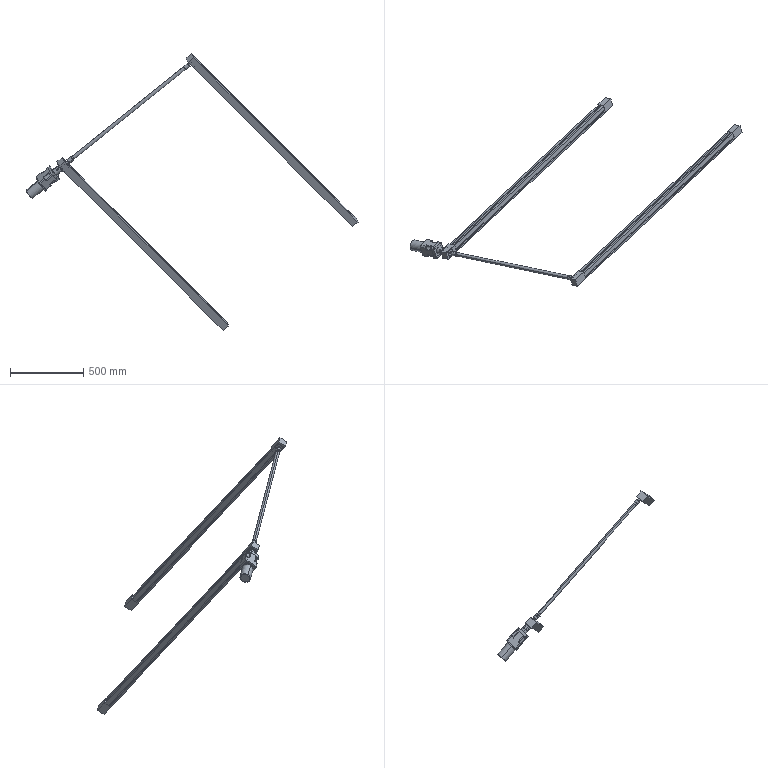Part | SolidWorks | 8 solids | 366 faces | box 2273 x 1295 x 1895 mm | volume 10477975 mm3 | cylinder 171 | plane 161 | cone 34 | commonest cylinder face diameters 5 x32 4.2 x24 6 x24 10 x12 116 x12 12 x10